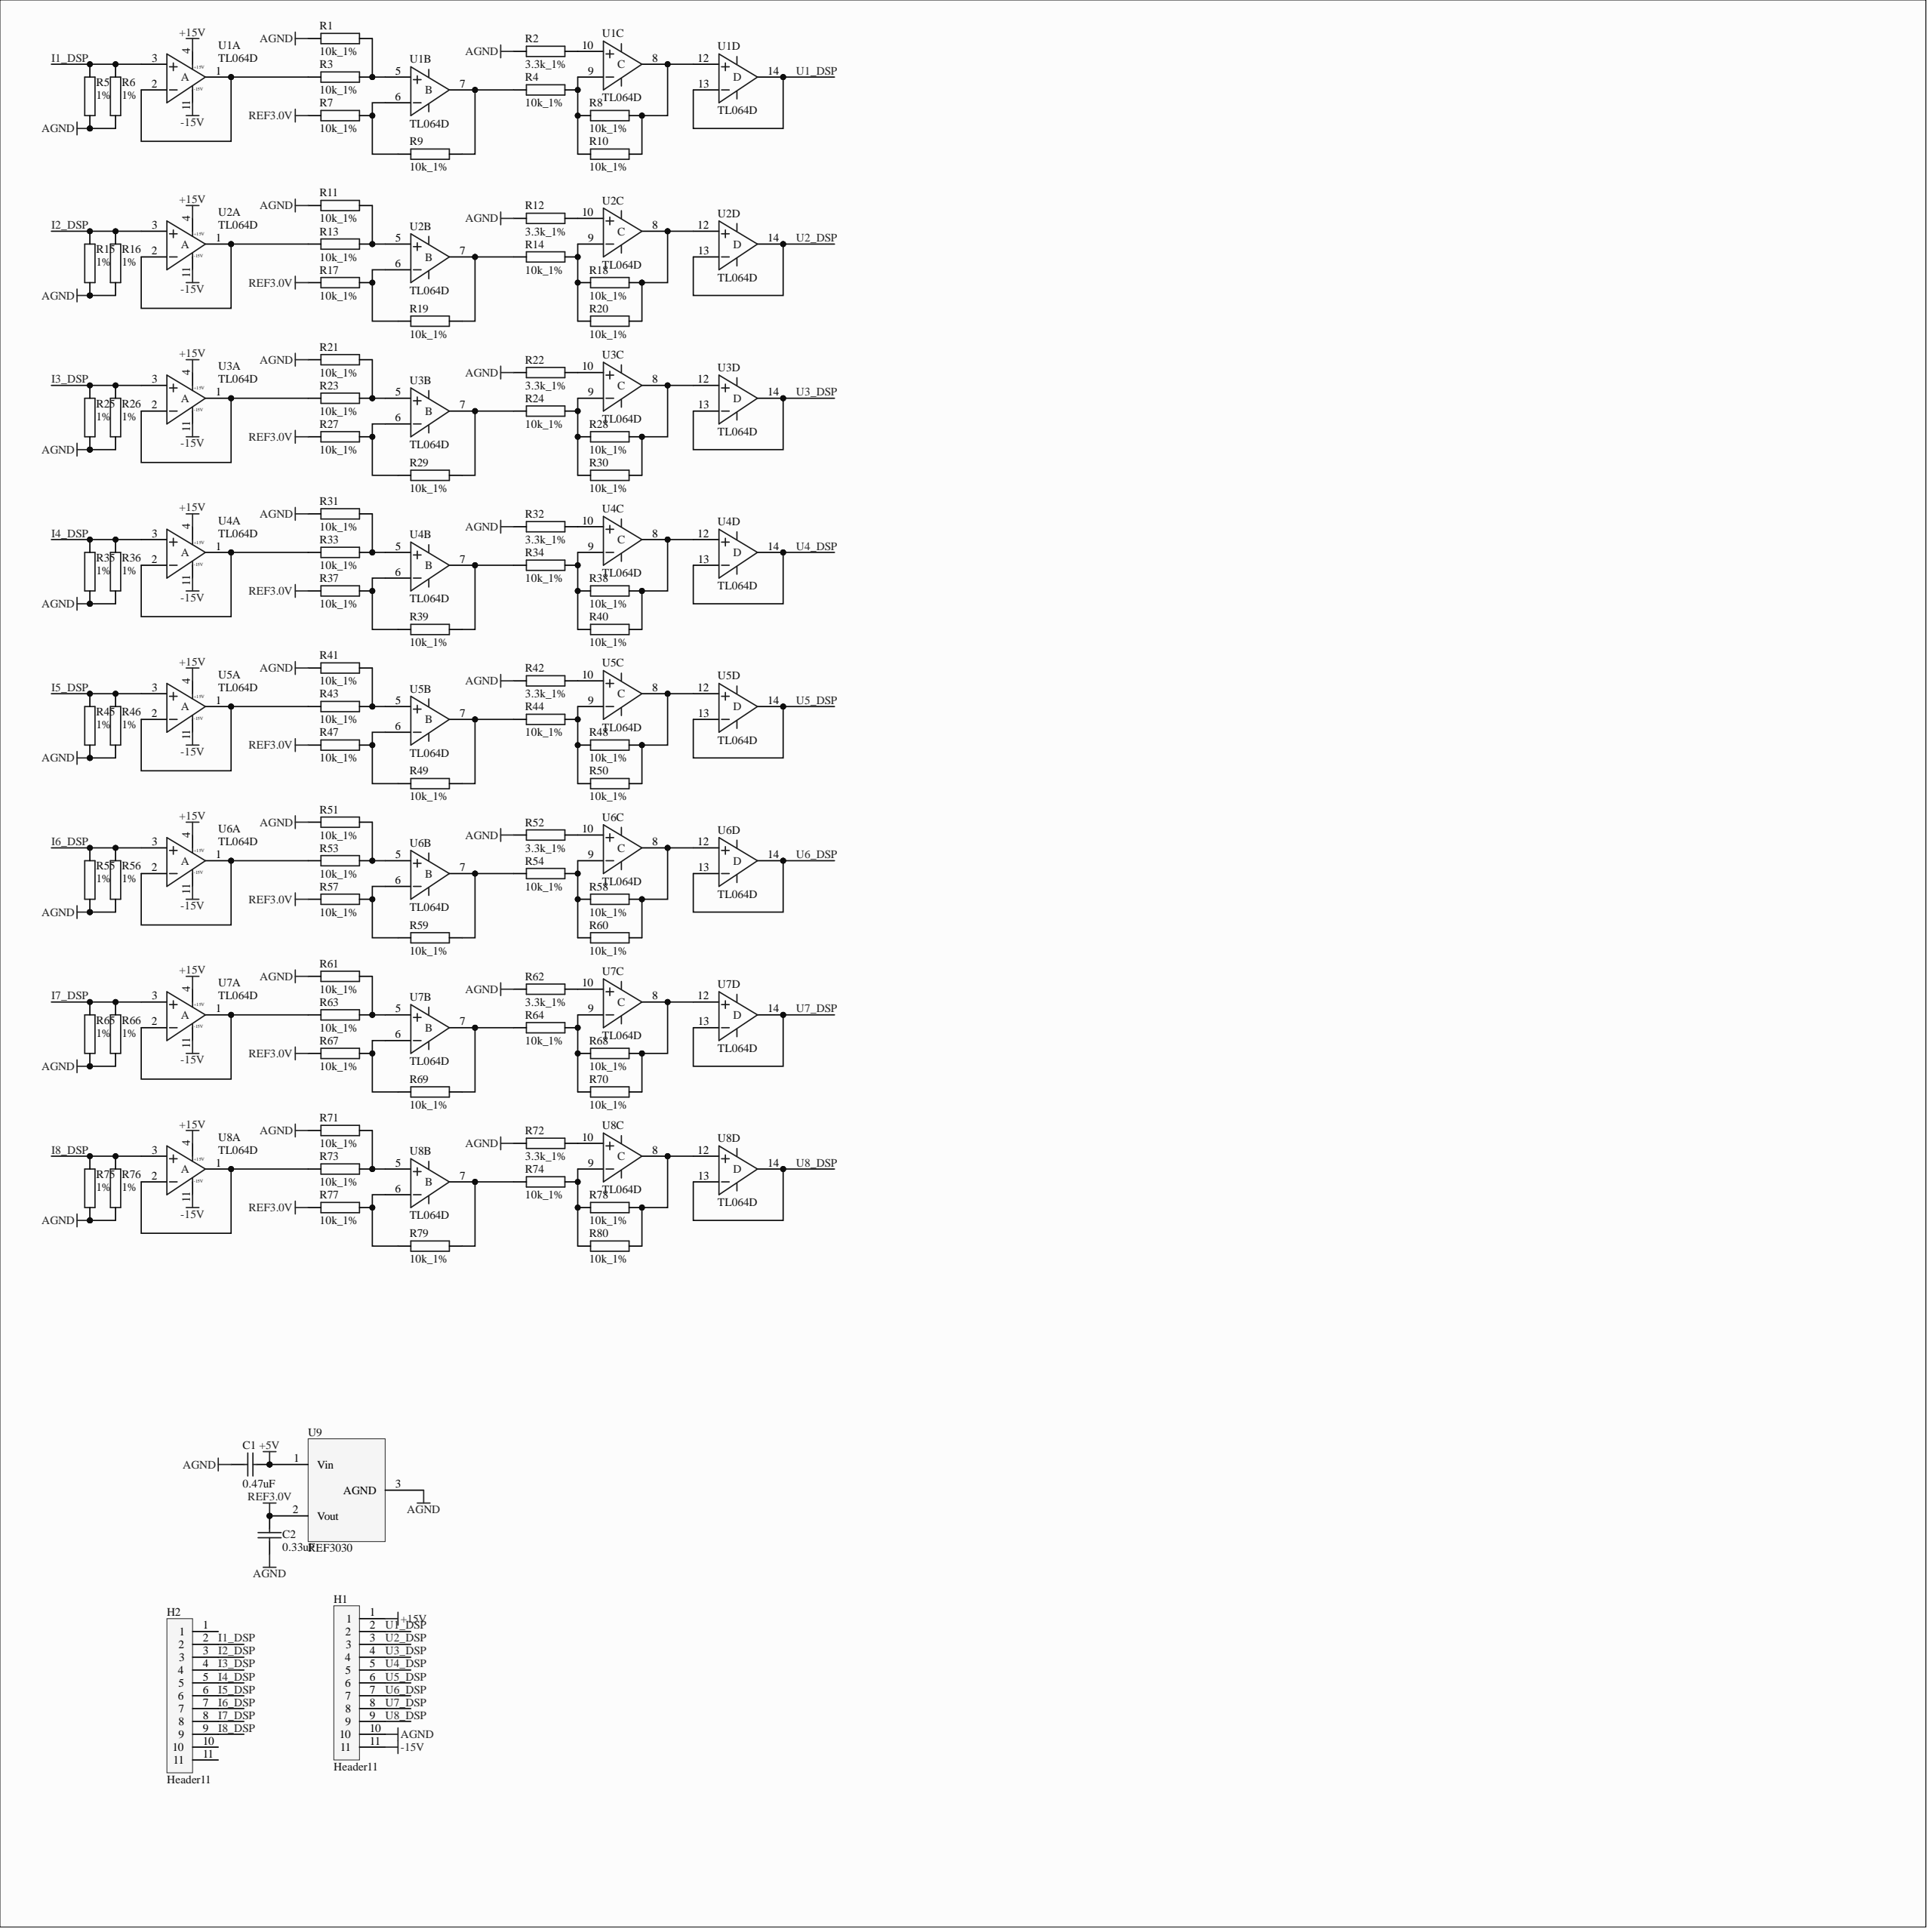Circuit board | Altium Designer | 93 parts | 77 nets
Bill of materials:
Comment,Description,Designator,Footprint,LibRef,Quantity
"0.47uF","Capacitor","C1","0603","CAP","1"
"0.33uF","Capacitor","C2","0603","CAP","1"
"Header11","Header11","H1, H2","PinHeader11_1.27mm","Header11","2"
"10k_1%","","R1, R3, R4, R7, R8, R9, R10, R11, R13, R14, R17, R18, R19, R20, R21, R23, R24, R27, R28, R29, R30, R31, R33, R34, R37, R38, R39, R40, R41, R43, R44, R47, R48, R49, R50, R51, R53, R54, R57, R58, R59, R60, R61, R63, R64, R67, R68, R69, R70, R71, R73, R74, R77, R78, R79, R80","0603","ProE260.TMP_300K_25","56"
"3.3k_1%","","R2, R12, R22, R32, R42, R52, R62, R72","0603","ProE260.TMP_300K_25","8"
"1%","","R5, R6, R15, R16, R25, R26, R35, R36, R45, R46, R55, R56, R65, R66, R75, R76","0805","ProE260.TMP_300K_25","16"
"TL064D","TI TL064D","U1, U2, U3, U4, U5, U6, U7, U8","TL064D_SOIC-14","TL064D","8"
"REF3030","","U9","SOT-23","REF3030","1"
Netlist (Protel format):
[
C1
0603
0.47uF



]
[
C2
0603
0.33uF



]
[
H1
PinHeader11_1.27mm
Header11



]
[
H2
PinHeader11_1.27mm
Header11



]
[
R1
0603
10k_1%



]
[
R2
0603
3.3k_1%



]
[
R3
0603
10k_1%



]
[
R4
0603
10k_1%



]
[
R5
0805
1%



]
[
R6
0805
1%



]
[
R7
0603
10k_1%



]
[
R8
0603
10k_1%



]
[
R9
0603
10k_1%



]
[
R10
0603
10k_1%



]
[
R11
0603
10k_1%



]
[
R12
0603
3.3k_1%



]
[
R13
0603
10k_1%



]
[
R14
0603
10k_1%



]
[
R15
0805
1%



]
[
R16
0805
1%



]
[
R17
0603
10k_1%



]
[
R18
0603
10k_1%



]
[
R19
0603
10k_1%



]
[
R20
0603
10k_1%



]
[
R21
0603
10k_1%



]
[
R22
0603
3.3k_1%



]
[
R23
0603
10k_1%



]
[
R24
0603
10k_1%



]
[
R25
0805
1%



]
[
R26
0805
1%



]
[
R27
0603
10k_1%



]
[
R28
0603
10k_1%



]
[
R29
0603
10k_1%



]
[
R30
0603
10k_1%



]
[
R31
0603
10k_1%



]
[
R32
0603
3.3k_1%



]
[
R33
0603
10k_1%



]
[
R34
0603
10k_1%



]
[
R35
0805
1%



]
[
R36
0805
1%



]
[
R37
0603
10k_1%



]
[
R38
0603
10k_1%



]
[
R39
0603
10k_1%



]
[
R40
0603
10k_1%



]
[
R41
0603
10k_1%



]
[
R42
0603
3.3k_1%



]
[
R43
0603
10k_1%



]
[
R44
0603
10k_1%



]
[
R45
0805
1%



]
[
R46
0805
1%



]
[
R47
0603
10k_1%



]
[
R48
0603
10k_1%



]
[
R49
0603
10k_1%



]
[
R50
0603
10k_1%



]
[
R51
0603
10k_1%



]
[
R52
0603
3.3k_1%



]
[
R53
0603
10k_1%



]
[
R54
0603
10k_1%



]
[
R55
0805
1%



]
[
R56
0805
1%



]
[
R57
0603
10k_1%



]
[
R58
0603
10k_1%



]
[
R59
0603
10k_1%



]
[
R60
0603
10k_1%



]
[
R61
0603
10k_1%



]
[
R62
0603
3.3k_1%



]
[
R63
0603
10k_1%



]
[
R64
0603
10k_1%



]
[
R65
0805
1%



]
[
R66
0805
1%



]
[
R67
0603
10k_1%



]
[
R68
0603
10k_1%



]
[
R69
0603
10k_1%



]
[
R70
0603
10k_1%



]
[
R71
0603
10k_1%



]
[
R72
0603
3.3k_1%



]
[
R73
0603
10k_1%



]
[
R74
0603
10k_1%



]
[
R75
0805
1%



]
[
R76
0805
1%



]
[
R77
0603
10k_1%



]
[
R78
0603
10k_1%



]
[
R79
0603
10k_1%



]
[
R80
0603
10k_1%



]
[
U1
TL064D_SOIC-14
TL064D



]
[
U2
TL064D_SOIC-14
TL064D



]
[
U3
TL064D_SOIC-14
TL064D



]
[
U4
TL064D_SOIC-14
TL064D



]
[
U5
TL064D_SOIC-14
TL064D



]
[
U6
TL064D_SOIC-14
TL064D



]
[
U7
TL064D_SOIC-14
TL064D



]
[
U8
TL064D_SOIC-14
TL064D



]
[
U9
SOT-23
REF3030



]
(
U8_DSP
H1-9
U8-13
U8-14
)
(
U7_DSP
H1-8
U7-13
U7-14
)
(
U6_DSP
H1-7
U6-13
U6-14
)
(
U5_DSP
H1-6
U5-13
U5-14
)
(
U4_DSP
H1-5
U4-13
U4-14
)
(
U3_DSP
H1-4
U3-13
U3-14
)
(
U2_DSP
H1-3
U2-13
U2-14
)
(
U1_DSP
H1-2
U1-13
U1-14
)
(
REF3.0V
C2-1
R7-1
R17-1
R27-1
R37-1
R47-1
R57-1
R67-1
R77-1
U9-2
)
(
NetR78_2
R78-2
R80-2
U8-8
U8-12
)
(
NetR77_2
R77-2
R79-1
U8-6
)
(
NetR74_2
R74-2
R78-1
R80-1
U8-9
)
(
NetR74_1
R74-1
R79-2
U8-7
)
(
NetR73_1
R73-1
U8-1
U8-2
)
(
NetR72_2
R72-2
U8-10
)
(
NetR71_2
R71-2
R73-2
U8-5
)
(
NetR68_2
R68-2
R70-2
U7-8
U7-12
)
(
NetR67_2
R67-2
R69-1
U7-6
)
(
NetR64_2
R64-2
R68-1
R70-1
U7-9
)
(
NetR64_1
R64-1
R69-2
U7-7
)
(
NetR63_1
R63-1
U7-1
U7-2
)
(
NetR62_2
R62-2
U7-10
)
(
NetR61_2
R61-2
R63-2
U7-5
)
(
NetR58_2
R58-2
R60-2
U6-8
U6-12
)
(
NetR57_2
R57-2
R59-1
U6-6
)
(
NetR54_2
R54-2
R58-1
R60-1
U6-9
)
(
NetR54_1
R54-1
R59-2
U6-7
)
(
NetR53_1
R53-1
U6-1
U6-2
)
(
NetR52_2
R52-2
U6-10
)
(
NetR51_2
R51-2
R53-2
U6-5
)
(
NetR48_2
R48-2
R50-2
U5-8
U5-12
)
(
NetR47_2
R47-2
R49-1
U5-6
)
(
NetR44_2
R44-2
R48-1
R50-1
U5-9
)
(
NetR44_1
R44-1
R49-2
U5-7
)
(
NetR43_1
R43-1
U5-1
U5-2
)
(
NetR42_2
R42-2
U5-10
)
(
NetR41_2
R41-2
R43-2
U5-5
)
(
NetR38_2
R38-2
R40-2
U4-8
U4-12
)
(
NetR37_2
R37-2
R39-1
U4-6
)
(
NetR34_2
R34-2
R38-1
R40-1
U4-9
)
(
NetR34_1
R34-1
R39-2
U4-7
)
(
NetR33_1
R33-1
U4-1
U4-2
)
(
NetR32_2
R32-2
U4-10
)
(
NetR31_2
R31-2
R33-2
U4-5
)
(
NetR28_2
R28-2
R30-2
U3-8
U3-12
)
(
NetR27_2
R27-2
R29-1
U3-6
)
(
NetR24_2
R24-2
R28-1
R30-1
U3-9
)
(
NetR24_1
R24-1
R29-2
U3-7
)
(
NetR23_1
R23-1
U3-1
U3-2
)
(
NetR22_2
R22-2
U3-10
)
(
NetR21_2
R21-2
R23-2
U3-5
)
(
NetR18_2
R18-2
R20-2
U2-8
U2-12
)
(
NetR17_2
R17-2
R19-1
U2-6
)
(
NetR14_2
R14-2
R18-1
R20-1
U2-9
)
(
NetR14_1
R14-1
R19-2
U2-7
)
(
NetR13_1
R13-1
U2-1
U2-2
)
(
NetR12_2
R12-2
U2-10
)
(
NetR11_2
R11-2
R13-2
U2-5
)
(
NetR8_2
R8-2
R10-2
U1-8
U1-12
)
(
NetR7_2
R7-2
R9-1
U1-6
)
(
NetR4_2
R4-2
R8-1
R10-1
U1-9
)
(
NetR4_1
R4-1
R9-2
U1-7
)
(
NetR3_1
R3-1
U1-1
U1-2
)
(
NetR2_2
R2-2
U1-10
)
(
NetR1_2
R1-2
R3-2
U1-5
)
(
I8_DSP
H2-9
R75-1
R76-1
U8-3
)
(
I7_DSP
H2-8
R65-1
R66-1
U7-3
)
(
I6_DSP
H2-7
R55-1
R56-1
U6-3
)
(
I5_DSP
H2-6
R45-1
R46-1
U5-3
)
(
I4_DSP
H2-5
R35-1
R36-1
U4-3
)
(
I3_DSP
H2-4
R25-1
R26-1
U3-3
)
(
I2_DSP
H2-3
R15-1
R16-1
U2-3
)
(
I1_DSP
H2-2
R5-1
R6-1
U1-3
)
(
AGND
C1-2
C2-2
H1-10
R1-1
R2-1
R5-2
R6-2
R11-1
R12-1
R15-2
R16-2
R21-1
R22-1
R25-2
R26-2
R31-1
R32-1
R35-2
R36-2
R41-1
R42-1
R45-2
R46-2
R51-1
R52-1
R55-2
R56-2
R61-1
R62-1
R65-2
R66-2
R71-1
R72-1
R75-2
R76-2
U9-3
)
(
-15V
H1-11
U1-11
U2-11
U3-11
U4-11
U5-11
U6-11
U7-11
U8-11
)
(
+15V
H1-1
U1-4
U2-4
U3-4
U4-4
U5-4
U6-4
U7-4
U8-4
)
(
+5V
C1-1
U9-1
)